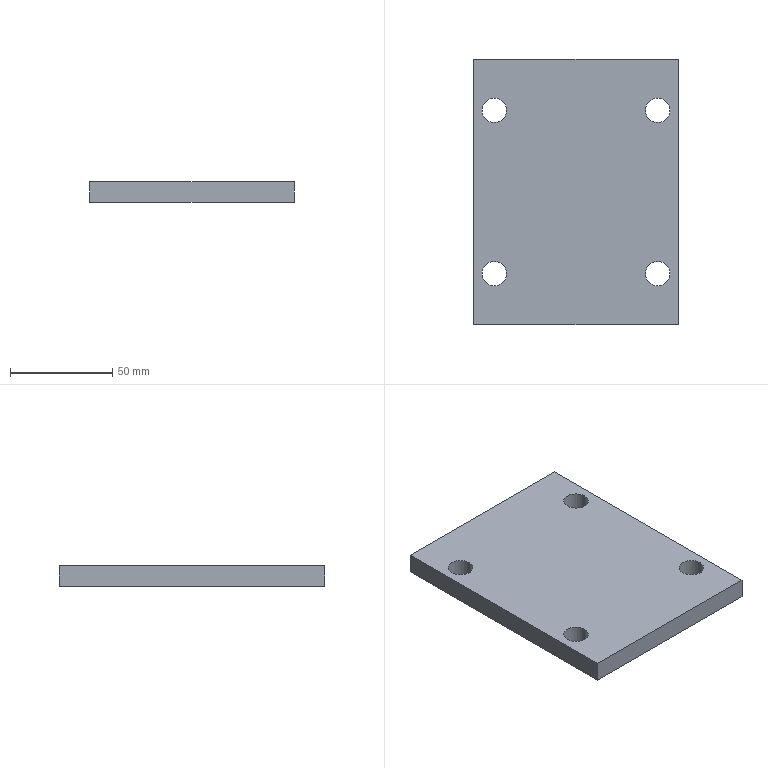Part | SolidWorks | features Chamfer 1, Extrusion 1, HoleWzd 1 | 1 solid | 14 faces | box 100 x 130 x 10 mm | volume 125476 mm3 | cylinder 8 | plane 6 | commonest cylinder face diameters 12 x8
STEP:
#1=CARTESIAN_POINT('',(-46.,40.,-5.));
#2=VERTEX_POINT('',#1);
#3=CARTESIAN_POINT('',(-34.,40.,-5.));
#4=VERTEX_POINT('',#3);
#5=CARTESIAN_POINT('',(-40.,40.,-5.));
#6=DIRECTION('',(0.,0.,1.));
#7=DIRECTION('',(1.,0.,0.));
#8=AXIS2_PLACEMENT_3D('',#5,#6,#7);
#9=CIRCLE('',#8,6.);
#10=EDGE_CURVE('',#2,#4,#9,.T.);
#11=ORIENTED_EDGE('',*,*,#10,.F.);
#12=CARTESIAN_POINT('',(-46.,40.,5.));
#13=VERTEX_POINT('',#12);
#14=CARTESIAN_POINT('',(-46.,40.,5.));
#15=DIRECTION('',(0.,0.,1.));
#16=VECTOR('',#15,1000.);
#17=LINE('',#14,#16);
#18=EDGE_CURVE('',#2,#13,#17,.T.);
#19=ORIENTED_EDGE('',*,*,#18,.T.);
#20=CARTESIAN_POINT('',(-34.,40.,5.));
#21=VERTEX_POINT('',#20);
#22=CARTESIAN_POINT('',(-40.,40.,5.));
#23=DIRECTION('',(0.,0.,1.));
#24=DIRECTION('',(1.,0.,0.));
#25=AXIS2_PLACEMENT_3D('',#22,#23,#24);
#26=CIRCLE('',#25,6.);
#27=EDGE_CURVE('',#13,#21,#26,.T.);
#28=ORIENTED_EDGE('',*,*,#27,.T.);
#29=CARTESIAN_POINT('',(-34.,40.,5.));
#30=DIRECTION('',(0.,0.,1.));
#31=VECTOR('',#30,1000.);
#32=LINE('',#29,#31);
#33=EDGE_CURVE('',#4,#21,#32,.T.);
#34=ORIENTED_EDGE('',*,*,#33,.F.);
#35=EDGE_LOOP('',(#11,#19,#28,#34));
#36=FACE_OUTER_BOUND('',#35,.T.);
#37=CARTESIAN_POINT('',(-40.,40.,5.));
#38=DIRECTION('',(0.,0.,1.));
#39=DIRECTION('',(1.,0.,0.));
#40=AXIS2_PLACEMENT_3D('',#37,#38,#39);
#41=CYLINDRICAL_SURFACE('',#40,6.);
#42=ADVANCED_FACE('',(#36),#41,.F.);
#43=CARTESIAN_POINT('',(34.,40.,-5.));
#44=VERTEX_POINT('',#43);
#45=CARTESIAN_POINT('',(46.,40.,-5.));
#46=VERTEX_POINT('',#45);
#47=CARTESIAN_POINT('',(40.,40.,-5.));
#48=DIRECTION('',(0.,0.,1.));
#49=DIRECTION('',(1.,0.,0.));
#50=AXIS2_PLACEMENT_3D('',#47,#48,#49);
#51=CIRCLE('',#50,6.);
#52=EDGE_CURVE('',#44,#46,#51,.T.);
#53=ORIENTED_EDGE('',*,*,#52,.F.);
#54=CARTESIAN_POINT('',(34.,40.,5.));
#55=VERTEX_POINT('',#54);
#56=CARTESIAN_POINT('',(34.,40.,5.));
#57=DIRECTION('',(0.,0.,1.));
#58=VECTOR('',#57,1000.);
#59=LINE('',#56,#58);
#60=EDGE_CURVE('',#44,#55,#59,.T.);
#61=ORIENTED_EDGE('',*,*,#60,.T.);
#62=CARTESIAN_POINT('',(46.,40.,5.));
#63=VERTEX_POINT('',#62);
#64=CARTESIAN_POINT('',(40.,40.,5.));
#65=DIRECTION('',(0.,0.,1.));
#66=DIRECTION('',(1.,0.,0.));
#67=AXIS2_PLACEMENT_3D('',#64,#65,#66);
#68=CIRCLE('',#67,6.);
#69=EDGE_CURVE('',#55,#63,#68,.T.);
#70=ORIENTED_EDGE('',*,*,#69,.T.);
#71=CARTESIAN_POINT('',(46.,40.,5.));
#72=DIRECTION('',(0.,0.,1.));
#73=VECTOR('',#72,1000.);
#74=LINE('',#71,#73);
#75=EDGE_CURVE('',#46,#63,#74,.T.);
#76=ORIENTED_EDGE('',*,*,#75,.F.);
#77=EDGE_LOOP('',(#53,#61,#70,#76));
#78=FACE_OUTER_BOUND('',#77,.T.);
#79=CARTESIAN_POINT('',(40.,40.,5.));
#80=DIRECTION('',(0.,0.,1.));
#81=DIRECTION('',(1.,0.,0.));
#82=AXIS2_PLACEMENT_3D('',#79,#80,#81);
#83=CYLINDRICAL_SURFACE('',#82,6.);
#84=ADVANCED_FACE('',(#78),#83,.F.);
#85=CARTESIAN_POINT('',(34.,-40.,-5.));
#86=VERTEX_POINT('',#85);
#87=CARTESIAN_POINT('',(46.,-40.,-5.));
#88=VERTEX_POINT('',#87);
#89=CARTESIAN_POINT('',(40.,-40.,-5.));
#90=DIRECTION('',(0.,0.,1.));
#91=DIRECTION('',(1.,0.,0.));
#92=AXIS2_PLACEMENT_3D('',#89,#90,#91);
#93=CIRCLE('',#92,6.);
#94=EDGE_CURVE('',#86,#88,#93,.T.);
#95=ORIENTED_EDGE('',*,*,#94,.F.);
#96=CARTESIAN_POINT('',(34.,-40.,5.));
#97=VERTEX_POINT('',#96);
#98=CARTESIAN_POINT('',(34.,-40.,5.));
#99=DIRECTION('',(0.,0.,1.));
#100=VECTOR('',#99,1000.);
#101=LINE('',#98,#100);
#102=EDGE_CURVE('',#86,#97,#101,.T.);
#103=ORIENTED_EDGE('',*,*,#102,.T.);
#104=CARTESIAN_POINT('',(46.,-40.,5.));
#105=VERTEX_POINT('',#104);
#106=CARTESIAN_POINT('',(40.,-40.,5.));
#107=DIRECTION('',(0.,0.,1.));
#108=DIRECTION('',(1.,0.,0.));
#109=AXIS2_PLACEMENT_3D('',#106,#107,#108);
#110=CIRCLE('',#109,6.);
#111=EDGE_CURVE('',#97,#105,#110,.T.);
#112=ORIENTED_EDGE('',*,*,#111,.T.);
#113=CARTESIAN_POINT('',(46.,-40.,5.));
#114=DIRECTION('',(0.,0.,1.));
#115=VECTOR('',#114,1000.);
#116=LINE('',#113,#115);
#117=EDGE_CURVE('',#88,#105,#116,.T.);
#118=ORIENTED_EDGE('',*,*,#117,.F.);
#119=EDGE_LOOP('',(#95,#103,#112,#118));
#120=FACE_OUTER_BOUND('',#119,.T.);
#121=CARTESIAN_POINT('',(40.,-40.,5.));
#122=DIRECTION('',(0.,0.,1.));
#123=DIRECTION('',(1.,0.,0.));
#124=AXIS2_PLACEMENT_3D('',#121,#122,#123);
#125=CYLINDRICAL_SURFACE('',#124,6.);
#126=ADVANCED_FACE('',(#120),#125,.F.);
#127=CARTESIAN_POINT('',(-46.,-40.,-5.));
#128=VERTEX_POINT('',#127);
#129=CARTESIAN_POINT('',(-34.,-40.,-5.));
#130=VERTEX_POINT('',#129);
#131=CARTESIAN_POINT('',(-40.,-40.,-5.));
#132=DIRECTION('',(0.,0.,1.));
#133=DIRECTION('',(1.,0.,0.));
#134=AXIS2_PLACEMENT_3D('',#131,#132,#133);
#135=CIRCLE('',#134,6.);
#136=EDGE_CURVE('',#128,#130,#135,.T.);
#137=ORIENTED_EDGE('',*,*,#136,.F.);
#138=CARTESIAN_POINT('',(-46.,-40.,5.));
#139=VERTEX_POINT('',#138);
#140=CARTESIAN_POINT('',(-46.,-40.,5.));
#141=DIRECTION('',(0.,0.,1.));
#142=VECTOR('',#141,1000.);
#143=LINE('',#140,#142);
#144=EDGE_CURVE('',#128,#139,#143,.T.);
#145=ORIENTED_EDGE('',*,*,#144,.T.);
#146=CARTESIAN_POINT('',(-34.,-40.,5.));
#147=VERTEX_POINT('',#146);
#148=CARTESIAN_POINT('',(-40.,-40.,5.));
#149=DIRECTION('',(0.,0.,1.));
#150=DIRECTION('',(1.,0.,0.));
#151=AXIS2_PLACEMENT_3D('',#148,#149,#150);
#152=CIRCLE('',#151,6.);
#153=EDGE_CURVE('',#139,#147,#152,.T.);
#154=ORIENTED_EDGE('',*,*,#153,.T.);
#155=CARTESIAN_POINT('',(-34.,-40.,5.));
#156=DIRECTION('',(0.,0.,1.));
#157=VECTOR('',#156,1000.);
#158=LINE('',#155,#157);
#159=EDGE_CURVE('',#130,#147,#158,.T.);
#160=ORIENTED_EDGE('',*,*,#159,.F.);
#161=EDGE_LOOP('',(#137,#145,#154,#160));
#162=FACE_OUTER_BOUND('',#161,.T.);
#163=CARTESIAN_POINT('',(-40.,-40.,5.));
#164=DIRECTION('',(0.,0.,1.));
#165=DIRECTION('',(1.,0.,0.));
#166=AXIS2_PLACEMENT_3D('',#163,#164,#165);
#167=CYLINDRICAL_SURFACE('',#166,6.);
#168=ADVANCED_FACE('',(#162),#167,.F.);
#169=CARTESIAN_POINT('',(-50.,65.,-5.));
#170=VERTEX_POINT('',#169);
#171=CARTESIAN_POINT('',(-50.,-65.,-5.));
#172=VERTEX_POINT('',#171);
#173=CARTESIAN_POINT('',(-50.,-65.,-5.));
#174=DIRECTION('',(0.,-1.,0.));
#175=VECTOR('',#174,1000.);
#176=LINE('',#173,#175);
#177=EDGE_CURVE('',#170,#172,#176,.T.);
#178=ORIENTED_EDGE('',*,*,#177,.T.);
#179=CARTESIAN_POINT('',(-50.,-65.,5.));
#180=VERTEX_POINT('',#179);
#181=CARTESIAN_POINT('',(-50.,-65.,5.));
#182=DIRECTION('',(0.,0.,-1.));
#183=VECTOR('',#182,1000.);
#184=LINE('',#181,#183);
#185=EDGE_CURVE('',#180,#172,#184,.T.);
#186=ORIENTED_EDGE('',*,*,#185,.F.);
#187=CARTESIAN_POINT('',(-50.,65.,5.));
#188=VERTEX_POINT('',#187);
#189=CARTESIAN_POINT('',(-50.,-65.,5.));
#190=DIRECTION('',(0.,-1.,0.));
#191=VECTOR('',#190,1000.);
#192=LINE('',#189,#191);
#193=EDGE_CURVE('',#188,#180,#192,.T.);
#194=ORIENTED_EDGE('',*,*,#193,.F.);
#195=CARTESIAN_POINT('',(-50.,65.,5.));
#196=DIRECTION('',(0.,0.,-1.));
#197=VECTOR('',#196,1000.);
#198=LINE('',#195,#197);
#199=EDGE_CURVE('',#188,#170,#198,.T.);
#200=ORIENTED_EDGE('',*,*,#199,.T.);
#201=EDGE_LOOP('',(#178,#186,#194,#200));
#202=FACE_OUTER_BOUND('',#201,.T.);
#203=CARTESIAN_POINT('',(-50.,-65.,5.));
#204=DIRECTION('',(1.,0.,0.));
#205=DIRECTION('',(0.,0.,-1.));
#206=AXIS2_PLACEMENT_3D('',#203,#204,#205);
#207=PLANE('',#206);
#208=ADVANCED_FACE('',(#202),#207,.F.);
#209=CARTESIAN_POINT('',(50.,-65.,-5.));
#210=VERTEX_POINT('',#209);
#211=CARTESIAN_POINT('',(50.,-65.,-5.));
#212=DIRECTION('',(1.,0.,0.));
#213=VECTOR('',#212,1000.);
#214=LINE('',#211,#213);
#215=EDGE_CURVE('',#172,#210,#214,.T.);
#216=ORIENTED_EDGE('',*,*,#215,.T.);
#217=CARTESIAN_POINT('',(50.,-65.,5.));
#218=VERTEX_POINT('',#217);
#219=CARTESIAN_POINT('',(50.,-65.,5.));
#220=DIRECTION('',(0.,0.,-1.));
#221=VECTOR('',#220,1000.);
#222=LINE('',#219,#221);
#223=EDGE_CURVE('',#218,#210,#222,.T.);
#224=ORIENTED_EDGE('',*,*,#223,.F.);
#225=CARTESIAN_POINT('',(50.,-65.,5.));
#226=DIRECTION('',(1.,0.,0.));
#227=VECTOR('',#226,1000.);
#228=LINE('',#225,#227);
#229=EDGE_CURVE('',#180,#218,#228,.T.);
#230=ORIENTED_EDGE('',*,*,#229,.F.);
#231=ORIENTED_EDGE('',*,*,#185,.T.);
#232=EDGE_LOOP('',(#216,#224,#230,#231));
#233=FACE_OUTER_BOUND('',#232,.T.);
#234=CARTESIAN_POINT('',(50.,-65.,5.));
#235=DIRECTION('',(0.,1.,0.));
#236=DIRECTION('',(-1.,0.,0.));
#237=AXIS2_PLACEMENT_3D('',#234,#235,#236);
#238=PLANE('',#237);
#239=ADVANCED_FACE('',(#233),#238,.F.);
#240=CARTESIAN_POINT('',(50.,65.,-5.));
#241=VERTEX_POINT('',#240);
#242=CARTESIAN_POINT('',(50.,-65.,-5.));
#243=DIRECTION('',(0.,1.,0.));
#244=VECTOR('',#243,1000.);
#245=LINE('',#242,#244);
#246=EDGE_CURVE('',#210,#241,#245,.T.);
#247=ORIENTED_EDGE('',*,*,#246,.T.);
#248=CARTESIAN_POINT('',(50.,65.,5.));
#249=VERTEX_POINT('',#248);
#250=CARTESIAN_POINT('',(50.,65.,5.));
#251=DIRECTION('',(0.,0.,-1.));
#252=VECTOR('',#251,1000.);
#253=LINE('',#250,#252);
#254=EDGE_CURVE('',#249,#241,#253,.T.);
#255=ORIENTED_EDGE('',*,*,#254,.F.);
#256=CARTESIAN_POINT('',(50.,-65.,5.));
#257=DIRECTION('',(0.,1.,0.));
#258=VECTOR('',#257,1000.);
#259=LINE('',#256,#258);
#260=EDGE_CURVE('',#218,#249,#259,.T.);
#261=ORIENTED_EDGE('',*,*,#260,.F.);
#262=ORIENTED_EDGE('',*,*,#223,.T.);
#263=EDGE_LOOP('',(#247,#255,#261,#262));
#264=FACE_OUTER_BOUND('',#263,.T.);
#265=CARTESIAN_POINT('',(50.,-65.,5.));
#266=DIRECTION('',(-1.,0.,0.));
#267=DIRECTION('',(0.,0.,1.));
#268=AXIS2_PLACEMENT_3D('',#265,#266,#267);
#269=PLANE('',#268);
#270=ADVANCED_FACE('',(#264),#269,.F.);
#271=CARTESIAN_POINT('',(50.,65.,-5.));
#272=DIRECTION('',(-1.,0.,0.));
#273=VECTOR('',#272,1000.);
#274=LINE('',#271,#273);
#275=EDGE_CURVE('',#241,#170,#274,.T.);
#276=ORIENTED_EDGE('',*,*,#275,.T.);
#277=ORIENTED_EDGE('',*,*,#199,.F.);
#278=CARTESIAN_POINT('',(50.,65.,5.));
#279=DIRECTION('',(-1.,0.,0.));
#280=VECTOR('',#279,1000.);
#281=LINE('',#278,#280);
#282=EDGE_CURVE('',#249,#188,#281,.T.);
#283=ORIENTED_EDGE('',*,*,#282,.F.);
#284=ORIENTED_EDGE('',*,*,#254,.T.);
#285=EDGE_LOOP('',(#276,#277,#283,#284));
#286=FACE_OUTER_BOUND('',#285,.T.);
#287=CARTESIAN_POINT('',(50.,65.,5.));
#288=DIRECTION('',(0.,-1.,0.));
#289=DIRECTION('',(0.,0.,-1.));
#290=AXIS2_PLACEMENT_3D('',#287,#288,#289);
#291=PLANE('',#290);
#292=ADVANCED_FACE('',(#286),#291,.F.);
#293=CARTESIAN_POINT('',(-40.,40.,5.));
#294=DIRECTION('',(0.,0.,1.));
#295=DIRECTION('',(1.,0.,0.));
#296=AXIS2_PLACEMENT_3D('',#293,#294,#295);
#297=CIRCLE('',#296,6.);
#298=EDGE_CURVE('',#21,#13,#297,.T.);
#299=ORIENTED_EDGE('',*,*,#298,.F.);
#300=ORIENTED_EDGE('',*,*,#27,.F.);
#301=EDGE_LOOP('',(#299,#300));
#302=FACE_BOUND('',#301,.T.);
#303=CARTESIAN_POINT('',(40.,40.,5.));
#304=DIRECTION('',(0.,0.,1.));
#305=DIRECTION('',(1.,0.,0.));
#306=AXIS2_PLACEMENT_3D('',#303,#304,#305);
#307=CIRCLE('',#306,6.);
#308=EDGE_CURVE('',#63,#55,#307,.T.);
#309=ORIENTED_EDGE('',*,*,#308,.F.);
#310=ORIENTED_EDGE('',*,*,#69,.F.);
#311=EDGE_LOOP('',(#309,#310));
#312=FACE_BOUND('',#311,.T.);
#313=CARTESIAN_POINT('',(40.,-40.,5.));
#314=DIRECTION('',(0.,0.,1.));
#315=DIRECTION('',(1.,0.,0.));
#316=AXIS2_PLACEMENT_3D('',#313,#314,#315);
#317=CIRCLE('',#316,6.);
#318=EDGE_CURVE('',#105,#97,#317,.T.);
#319=ORIENTED_EDGE('',*,*,#318,.F.);
#320=ORIENTED_EDGE('',*,*,#111,.F.);
#321=EDGE_LOOP('',(#319,#320));
#322=FACE_BOUND('',#321,.T.);
#323=CARTESIAN_POINT('',(-40.,-40.,5.));
#324=DIRECTION('',(0.,0.,1.));
#325=DIRECTION('',(1.,0.,0.));
#326=AXIS2_PLACEMENT_3D('',#323,#324,#325);
#327=CIRCLE('',#326,6.);
#328=EDGE_CURVE('',#147,#139,#327,.T.);
#329=ORIENTED_EDGE('',*,*,#328,.F.);
#330=ORIENTED_EDGE('',*,*,#153,.F.);
#331=EDGE_LOOP('',(#329,#330));
#332=FACE_BOUND('',#331,.T.);
#333=ORIENTED_EDGE('',*,*,#193,.T.);
#334=ORIENTED_EDGE('',*,*,#229,.T.);
#335=ORIENTED_EDGE('',*,*,#260,.T.);
#336=ORIENTED_EDGE('',*,*,#282,.T.);
#337=EDGE_LOOP('',(#333,#334,#335,#336));
#338=FACE_OUTER_BOUND('',#337,.T.);
#339=CARTESIAN_POINT('',(0.,0.,5.));
#340=DIRECTION('',(0.,0.,1.));
#341=DIRECTION('',(1.,0.,0.));
#342=AXIS2_PLACEMENT_3D('',#339,#340,#341);
#343=PLANE('',#342);
#344=ADVANCED_FACE('',(#302,#312,#322,#332,#338),#343,.T.);
#345=CARTESIAN_POINT('',(-40.,40.,-5.));
#346=DIRECTION('',(0.,0.,1.));
#347=DIRECTION('',(1.,0.,0.));
#348=AXIS2_PLACEMENT_3D('',#345,#346,#347);
#349=CIRCLE('',#348,6.);
#350=EDGE_CURVE('',#4,#2,#349,.T.);
#351=ORIENTED_EDGE('',*,*,#350,.T.);
#352=ORIENTED_EDGE('',*,*,#10,.T.);
#353=EDGE_LOOP('',(#351,#352));
#354=FACE_BOUND('',#353,.T.);
#355=CARTESIAN_POINT('',(40.,40.,-5.));
#356=DIRECTION('',(0.,0.,1.));
#357=DIRECTION('',(1.,0.,0.));
#358=AXIS2_PLACEMENT_3D('',#355,#356,#357);
#359=CIRCLE('',#358,6.);
#360=EDGE_CURVE('',#46,#44,#359,.T.);
#361=ORIENTED_EDGE('',*,*,#360,.T.);
#362=ORIENTED_EDGE('',*,*,#52,.T.);
#363=EDGE_LOOP('',(#361,#362));
#364=FACE_BOUND('',#363,.T.);
#365=CARTESIAN_POINT('',(40.,-40.,-5.));
#366=DIRECTION('',(0.,0.,1.));
#367=DIRECTION('',(1.,0.,0.));
#368=AXIS2_PLACEMENT_3D('',#365,#366,#367);
#369=CIRCLE('',#368,6.);
#370=EDGE_CURVE('',#88,#86,#369,.T.);
#371=ORIENTED_EDGE('',*,*,#370,.T.);
#372=ORIENTED_EDGE('',*,*,#94,.T.);
#373=EDGE_LOOP('',(#371,#372));
#374=FACE_BOUND('',#373,.T.);
#375=CARTESIAN_POINT('',(-40.,-40.,-5.));
#376=DIRECTION('',(0.,0.,1.));
#377=DIRECTION('',(1.,0.,0.));
#378=AXIS2_PLACEMENT_3D('',#375,#376,#377);
#379=CIRCLE('',#378,6.);
#380=EDGE_CURVE('',#130,#128,#379,.T.);
#381=ORIENTED_EDGE('',*,*,#380,.T.);
#382=ORIENTED_EDGE('',*,*,#136,.T.);
#383=EDGE_LOOP('',(#381,#382));
#384=FACE_BOUND('',#383,.T.);
#385=ORIENTED_EDGE('',*,*,#177,.F.);
#386=ORIENTED_EDGE('',*,*,#275,.F.);
#387=ORIENTED_EDGE('',*,*,#246,.F.);
#388=ORIENTED_EDGE('',*,*,#215,.F.);
#389=EDGE_LOOP('',(#385,#386,#387,#388));
#390=FACE_OUTER_BOUND('',#389,.T.);
#391=CARTESIAN_POINT('',(0.,0.,-5.));
#392=DIRECTION('',(0.,0.,1.));
#393=DIRECTION('',(1.,0.,0.));
#394=AXIS2_PLACEMENT_3D('',#391,#392,#393);
#395=PLANE('',#394);
#396=ADVANCED_FACE('',(#354,#364,#374,#384,#390),#395,.F.);
#397=ORIENTED_EDGE('',*,*,#144,.F.);
#398=ORIENTED_EDGE('',*,*,#380,.F.);
#399=ORIENTED_EDGE('',*,*,#159,.T.);
#400=ORIENTED_EDGE('',*,*,#328,.T.);
#401=EDGE_LOOP('',(#397,#398,#399,#400));
#402=FACE_OUTER_BOUND('',#401,.T.);
#403=CARTESIAN_POINT('',(-40.,-40.,5.));
#404=DIRECTION('',(0.,0.,1.));
#405=DIRECTION('',(1.,0.,0.));
#406=AXIS2_PLACEMENT_3D('',#403,#404,#405);
#407=CYLINDRICAL_SURFACE('',#406,6.);
#408=ADVANCED_FACE('',(#402),#407,.F.);
#409=ORIENTED_EDGE('',*,*,#102,.F.);
#410=ORIENTED_EDGE('',*,*,#370,.F.);
#411=ORIENTED_EDGE('',*,*,#117,.T.);
#412=ORIENTED_EDGE('',*,*,#318,.T.);
#413=EDGE_LOOP('',(#409,#410,#411,#412));
#414=FACE_OUTER_BOUND('',#413,.T.);
#415=CARTESIAN_POINT('',(40.,-40.,5.));
#416=DIRECTION('',(0.,0.,1.));
#417=DIRECTION('',(1.,0.,0.));
#418=AXIS2_PLACEMENT_3D('',#415,#416,#417);
#419=CYLINDRICAL_SURFACE('',#418,6.);
#420=ADVANCED_FACE('',(#414),#419,.F.);
#421=ORIENTED_EDGE('',*,*,#60,.F.);
#422=ORIENTED_EDGE('',*,*,#360,.F.);
#423=ORIENTED_EDGE('',*,*,#75,.T.);
#424=ORIENTED_EDGE('',*,*,#308,.T.);
#425=EDGE_LOOP('',(#421,#422,#423,#424));
#426=FACE_OUTER_BOUND('',#425,.T.);
#427=CARTESIAN_POINT('',(40.,40.,5.));
#428=DIRECTION('',(0.,0.,1.));
#429=DIRECTION('',(1.,0.,0.));
#430=AXIS2_PLACEMENT_3D('',#427,#428,#429);
#431=CYLINDRICAL_SURFACE('',#430,6.);
#432=ADVANCED_FACE('',(#426),#431,.F.);
#433=ORIENTED_EDGE('',*,*,#18,.F.);
#434=ORIENTED_EDGE('',*,*,#350,.F.);
#435=ORIENTED_EDGE('',*,*,#33,.T.);
#436=ORIENTED_EDGE('',*,*,#298,.T.);
#437=EDGE_LOOP('',(#433,#434,#435,#436));
#438=FACE_OUTER_BOUND('',#437,.T.);
#439=CARTESIAN_POINT('',(-40.,40.,5.));
#440=DIRECTION('',(0.,0.,1.));
#441=DIRECTION('',(1.,0.,0.));
#442=AXIS2_PLACEMENT_3D('',#439,#440,#441);
#443=CYLINDRICAL_SURFACE('',#442,6.);
#444=ADVANCED_FACE('',(#438),#443,.F.);
#445=CLOSED_SHELL('',(#42,#84,#126,#168,#208,#239,#270,#292,#344,#396,#408,#420,#432,#444));
#446=MANIFOLD_SOLID_BREP('',#445);
#447=CARTESIAN_POINT('',(0.,0.,0.));
#448=DIRECTION('',(0.,0.,1.));
#449=DIRECTION('',(1.,0.,0.));
#450=AXIS2_PLACEMENT_3D('',#447,#448,#449);
#451=(LENGTH_UNIT()NAMED_UNIT(*)SI_UNIT(.MILLI.,.METRE.));
#452=UNCERTAINTY_MEASURE_WITH_UNIT(LENGTH_MEASURE(0.00001),#451,'','');
#453=(NAMED_UNIT(*)PLANE_ANGLE_UNIT()SI_UNIT($,.RADIAN.));
#454=(NAMED_UNIT(*)SI_UNIT($,.STERADIAN.)SOLID_ANGLE_UNIT());
#455=(GEOMETRIC_REPRESENTATION_CONTEXT(3)GLOBAL_UNCERTAINTY_ASSIGNED_CONTEXT((#452))GLOBAL_UNIT_ASSIGNED_CONTEXT((#451,#453,#454))REPRESENTATION_CONTEXT('',''));
#456=ADVANCED_BREP_SHAPE_REPRESENTATION('',(#446,#450),#455);